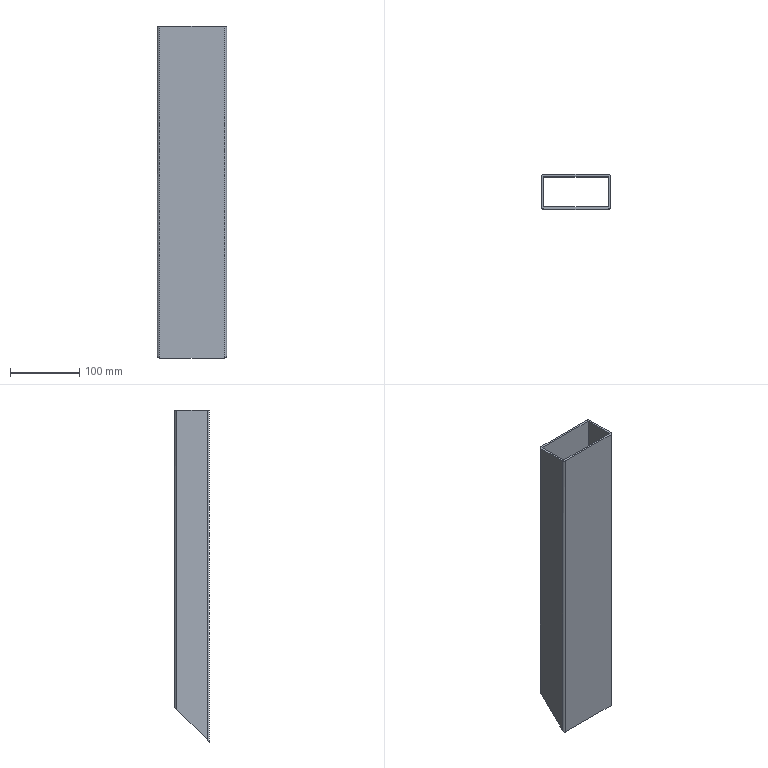Part | SolidWorks | features Extrusion 1, ICE 1 | 1 solid | 18 faces | box 100 x 50 x 480 mm | volume 389136 mm3 | plane 10 | cylinder 8 | commonest cylinder face diameters 0.4 x4 6.4 x4
STEP:
#1=CARTESIAN_POINT('',(-46.8,25.,500.));
#2=VERTEX_POINT('',#1);
#3=CARTESIAN_POINT('',(-46.8,25.,70.));
#4=VERTEX_POINT('',#3);
#5=CARTESIAN_POINT('',(-46.8,25.,500.));
#6=DIRECTION('',(0.,0.,-1.));
#7=VECTOR('',#6,1000.);
#8=LINE('',#5,#7);
#9=EDGE_CURVE('',#2,#4,#8,.T.);
#10=ORIENTED_EDGE('',*,*,#9,.T.);
#11=CARTESIAN_POINT('',(-50.,21.8,66.8));
#12=VERTEX_POINT('',#11);
#13=CARTESIAN_POINT('',(-46.8,25.,70.));
#14=CARTESIAN_POINT('',(-48.675,25.,70.));
#15=CARTESIAN_POINT('',(-50.,23.675,68.675));
#16=CARTESIAN_POINT('',(-50.,21.8,66.8));
#17=(BOUNDED_CURVE()B_SPLINE_CURVE(3,(#13,#14,#15,#16),.UNSPECIFIED.,.F.,.F.)B_SPLINE_CURVE_WITH_KNOTS((4,4),(3.142,4.712),.UNSPECIFIED.)CURVE()GEOMETRIC_REPRESENTATION_ITEM()RATIONAL_B_SPLINE_CURVE((1.,0.8047,0.8047,1.))REPRESENTATION_ITEM(''));
#18=EDGE_CURVE('',#4,#12,#17,.T.);
#19=ORIENTED_EDGE('',*,*,#18,.T.);
#20=CARTESIAN_POINT('',(-50.,21.8,500.));
#21=VERTEX_POINT('',#20);
#22=CARTESIAN_POINT('',(-50.,21.8,500.));
#23=DIRECTION('',(0.,0.,-1.));
#24=VECTOR('',#23,1000.);
#25=LINE('',#22,#24);
#26=EDGE_CURVE('',#21,#12,#25,.T.);
#27=ORIENTED_EDGE('',*,*,#26,.F.);
#28=CARTESIAN_POINT('',(-46.8,21.8,500.));
#29=DIRECTION('',(0.,0.,1.));
#30=DIRECTION('',(1.,0.,0.));
#31=AXIS2_PLACEMENT_3D('',#28,#29,#30);
#32=CIRCLE('',#31,3.2);
#33=EDGE_CURVE('',#2,#21,#32,.T.);
#34=ORIENTED_EDGE('',*,*,#33,.F.);
#35=EDGE_LOOP('',(#10,#19,#27,#34));
#36=FACE_OUTER_BOUND('',#35,.T.);
#37=CARTESIAN_POINT('',(-46.8,21.8,500.));
#38=DIRECTION('',(0.,0.,-1.));
#39=DIRECTION('',(-1.,0.,0.));
#40=AXIS2_PLACEMENT_3D('',#37,#38,#39);
#41=CYLINDRICAL_SURFACE('',#40,3.2);
#42=ADVANCED_FACE('',(#36),#41,.T.);
#43=ORIENTED_EDGE('',*,*,#26,.T.);
#44=CARTESIAN_POINT('',(-50.,-21.8,23.2));
#45=VERTEX_POINT('',#44);
#46=CARTESIAN_POINT('',(-50.,238.4,283.4));
#47=DIRECTION('',(0.,-0.7071,-0.7071));
#48=VECTOR('',#47,1000.);
#49=LINE('',#46,#48);
#50=EDGE_CURVE('',#12,#45,#49,.T.);
#51=ORIENTED_EDGE('',*,*,#50,.T.);
#52=CARTESIAN_POINT('',(-50.,-21.8,500.));
#53=VERTEX_POINT('',#52);
#54=CARTESIAN_POINT('',(-50.,-21.8,500.));
#55=DIRECTION('',(0.,0.,-1.));
#56=VECTOR('',#55,1000.);
#57=LINE('',#54,#56);
#58=EDGE_CURVE('',#53,#45,#57,.T.);
#59=ORIENTED_EDGE('',*,*,#58,.F.);
#60=CARTESIAN_POINT('',(-50.,21.8,500.));
#61=DIRECTION('',(0.,-1.,0.));
#62=VECTOR('',#61,1000.);
#63=LINE('',#60,#62);
#64=EDGE_CURVE('',#21,#53,#63,.T.);
#65=ORIENTED_EDGE('',*,*,#64,.F.);
#66=EDGE_LOOP('',(#43,#51,#59,#65));
#67=FACE_OUTER_BOUND('',#66,.T.);
#68=CARTESIAN_POINT('',(-50.,21.8,500.));
#69=DIRECTION('',(1.,0.,0.));
#70=DIRECTION('',(0.,1.,0.));
#71=AXIS2_PLACEMENT_3D('',#68,#69,#70);
#72=PLANE('',#71);
#73=ADVANCED_FACE('',(#67),#72,.F.);
#74=ORIENTED_EDGE('',*,*,#58,.T.);
#75=CARTESIAN_POINT('',(-46.8,-25.,20.));
#76=VERTEX_POINT('',#75);
#77=CARTESIAN_POINT('',(-50.,-21.8,23.2));
#78=CARTESIAN_POINT('',(-50.,-23.675,21.325));
#79=CARTESIAN_POINT('',(-48.675,-25.,20.));
#80=CARTESIAN_POINT('',(-46.8,-25.,20.));
#81=(BOUNDED_CURVE()B_SPLINE_CURVE(3,(#77,#78,#79,#80),.UNSPECIFIED.,.F.,.F.)B_SPLINE_CURVE_WITH_KNOTS((4,4),(4.712,6.283),.UNSPECIFIED.)CURVE()GEOMETRIC_REPRESENTATION_ITEM()RATIONAL_B_SPLINE_CURVE((1.,0.8047,0.8047,1.))REPRESENTATION_ITEM(''));
#82=EDGE_CURVE('',#45,#76,#81,.T.);
#83=ORIENTED_EDGE('',*,*,#82,.T.);
#84=CARTESIAN_POINT('',(-46.8,-25.,500.));
#85=VERTEX_POINT('',#84);
#86=CARTESIAN_POINT('',(-46.8,-25.,500.));
#87=DIRECTION('',(0.,0.,-1.));
#88=VECTOR('',#87,1000.);
#89=LINE('',#86,#88);
#90=EDGE_CURVE('',#85,#76,#89,.T.);
#91=ORIENTED_EDGE('',*,*,#90,.F.);
#92=CARTESIAN_POINT('',(-46.8,-21.8,500.));
#93=DIRECTION('',(0.,0.,1.));
#94=DIRECTION('',(1.,0.,0.));
#95=AXIS2_PLACEMENT_3D('',#92,#93,#94);
#96=CIRCLE('',#95,3.2);
#97=EDGE_CURVE('',#53,#85,#96,.T.);
#98=ORIENTED_EDGE('',*,*,#97,.F.);
#99=EDGE_LOOP('',(#74,#83,#91,#98));
#100=FACE_OUTER_BOUND('',#99,.T.);
#101=CARTESIAN_POINT('',(-46.8,-21.8,500.));
#102=DIRECTION('',(0.,0.,-1.));
#103=DIRECTION('',(-1.,0.,0.));
#104=AXIS2_PLACEMENT_3D('',#101,#102,#103);
#105=CYLINDRICAL_SURFACE('',#104,3.2);
#106=ADVANCED_FACE('',(#100),#105,.T.);
#107=ORIENTED_EDGE('',*,*,#90,.T.);
#108=CARTESIAN_POINT('',(46.8,-25.,20.));
#109=VERTEX_POINT('',#108);
#110=CARTESIAN_POINT('',(-430.,-25.,20.));
#111=DIRECTION('',(1.,0.,0.));
#112=VECTOR('',#111,1000.);
#113=LINE('',#110,#112);
#114=EDGE_CURVE('',#76,#109,#113,.T.);
#115=ORIENTED_EDGE('',*,*,#114,.T.);
#116=CARTESIAN_POINT('',(46.8,-25.,500.));
#117=VERTEX_POINT('',#116);
#118=CARTESIAN_POINT('',(46.8,-25.,500.));
#119=DIRECTION('',(0.,0.,-1.));
#120=VECTOR('',#119,1000.);
#121=LINE('',#118,#120);
#122=EDGE_CURVE('',#117,#109,#121,.T.);
#123=ORIENTED_EDGE('',*,*,#122,.F.);
#124=CARTESIAN_POINT('',(-46.8,-25.,500.));
#125=DIRECTION('',(1.,0.,0.));
#126=VECTOR('',#125,1000.);
#127=LINE('',#124,#126);
#128=EDGE_CURVE('',#85,#117,#127,.T.);
#129=ORIENTED_EDGE('',*,*,#128,.F.);
#130=EDGE_LOOP('',(#107,#115,#123,#129));
#131=FACE_OUTER_BOUND('',#130,.T.);
#132=CARTESIAN_POINT('',(-46.8,-25.,500.));
#133=DIRECTION('',(0.,1.,0.));
#134=DIRECTION('',(0.,0.,1.));
#135=AXIS2_PLACEMENT_3D('',#132,#133,#134);
#136=PLANE('',#135);
#137=ADVANCED_FACE('',(#131),#136,.F.);
#138=ORIENTED_EDGE('',*,*,#122,.T.);
#139=CARTESIAN_POINT('',(50.,-21.8,23.2));
#140=VERTEX_POINT('',#139);
#141=CARTESIAN_POINT('',(46.8,-25.,20.));
#142=CARTESIAN_POINT('',(48.675,-25.,20.));
#143=CARTESIAN_POINT('',(50.,-23.675,21.325));
#144=CARTESIAN_POINT('',(50.,-21.8,23.2));
#145=(BOUNDED_CURVE()B_SPLINE_CURVE(3,(#141,#142,#143,#144),.UNSPECIFIED.,.F.,.F.)B_SPLINE_CURVE_WITH_KNOTS((4,4),(0.,1.571),.UNSPECIFIED.)CURVE()GEOMETRIC_REPRESENTATION_ITEM()RATIONAL_B_SPLINE_CURVE((1.,0.8047,0.8047,1.))REPRESENTATION_ITEM(''));
#146=EDGE_CURVE('',#109,#140,#145,.T.);
#147=ORIENTED_EDGE('',*,*,#146,.T.);
#148=CARTESIAN_POINT('',(50.,-21.8,500.));
#149=VERTEX_POINT('',#148);
#150=CARTESIAN_POINT('',(50.,-21.8,500.));
#151=DIRECTION('',(0.,0.,-1.));
#152=VECTOR('',#151,1000.);
#153=LINE('',#150,#152);
#154=EDGE_CURVE('',#149,#140,#153,.T.);
#155=ORIENTED_EDGE('',*,*,#154,.F.);
#156=CARTESIAN_POINT('',(46.8,-21.8,500.));
#157=DIRECTION('',(0.,0.,1.));
#158=DIRECTION('',(1.,0.,0.));
#159=AXIS2_PLACEMENT_3D('',#156,#157,#158);
#160=CIRCLE('',#159,3.2);
#161=EDGE_CURVE('',#117,#149,#160,.T.);
#162=ORIENTED_EDGE('',*,*,#161,.F.);
#163=EDGE_LOOP('',(#138,#147,#155,#162));
#164=FACE_OUTER_BOUND('',#163,.T.);
#165=CARTESIAN_POINT('',(46.8,-21.8,500.));
#166=DIRECTION('',(0.,0.,-1.));
#167=DIRECTION('',(-1.,0.,0.));
#168=AXIS2_PLACEMENT_3D('',#165,#166,#167);
#169=CYLINDRICAL_SURFACE('',#168,3.2);
#170=ADVANCED_FACE('',(#164),#169,.T.);
#171=CARTESIAN_POINT('',(50.,21.8,66.8));
#172=VERTEX_POINT('',#171);
#173=CARTESIAN_POINT('',(50.,25.,70.));
#174=DIRECTION('',(0.,-0.7071,-0.7071));
#175=VECTOR('',#174,1000.);
#176=LINE('',#173,#175);
#177=EDGE_CURVE('',#172,#140,#176,.T.);
#178=ORIENTED_EDGE('',*,*,#177,.F.);
#179=CARTESIAN_POINT('',(50.,21.8,500.));
#180=VERTEX_POINT('',#179);
#181=CARTESIAN_POINT('',(50.,21.8,500.));
#182=DIRECTION('',(0.,0.,-1.));
#183=VECTOR('',#182,1000.);
#184=LINE('',#181,#183);
#185=EDGE_CURVE('',#180,#172,#184,.T.);
#186=ORIENTED_EDGE('',*,*,#185,.F.);
#187=CARTESIAN_POINT('',(50.,21.8,500.));
#188=DIRECTION('',(0.,-1.,0.));
#189=VECTOR('',#188,1000.);
#190=LINE('',#187,#189);
#191=EDGE_CURVE('',#180,#149,#190,.T.);
#192=ORIENTED_EDGE('',*,*,#191,.T.);
#193=ORIENTED_EDGE('',*,*,#154,.T.);
#194=EDGE_LOOP('',(#178,#186,#192,#193));
#195=FACE_OUTER_BOUND('',#194,.T.);
#196=CARTESIAN_POINT('',(50.,21.8,500.));
#197=DIRECTION('',(1.,0.,0.));
#198=DIRECTION('',(0.,1.,0.));
#199=AXIS2_PLACEMENT_3D('',#196,#197,#198);
#200=PLANE('',#199);
#201=ADVANCED_FACE('',(#195),#200,.T.);
#202=CARTESIAN_POINT('',(46.8,25.,70.));
#203=VERTEX_POINT('',#202);
#204=CARTESIAN_POINT('',(46.8,25.,70.));
#205=CARTESIAN_POINT('',(48.675,25.,70.));
#206=CARTESIAN_POINT('',(50.,23.675,68.675));
#207=CARTESIAN_POINT('',(50.,21.8,66.8));
#208=(BOUNDED_CURVE()B_SPLINE_CURVE(3,(#204,#205,#206,#207),.UNSPECIFIED.,.F.,.F.)B_SPLINE_CURVE_WITH_KNOTS((4,4),(3.142,4.712),.UNSPECIFIED.)CURVE()GEOMETRIC_REPRESENTATION_ITEM()RATIONAL_B_SPLINE_CURVE((1.,0.8047,0.8047,1.))REPRESENTATION_ITEM(''));
#209=EDGE_CURVE('',#203,#172,#208,.T.);
#210=ORIENTED_EDGE('',*,*,#209,.F.);
#211=CARTESIAN_POINT('',(46.8,25.,500.));
#212=VERTEX_POINT('',#211);
#213=CARTESIAN_POINT('',(46.8,25.,500.));
#214=DIRECTION('',(0.,0.,-1.));
#215=VECTOR('',#214,1000.);
#216=LINE('',#213,#215);
#217=EDGE_CURVE('',#212,#203,#216,.T.);
#218=ORIENTED_EDGE('',*,*,#217,.F.);
#219=CARTESIAN_POINT('',(46.8,21.8,500.));
#220=DIRECTION('',(0.,0.,-1.));
#221=DIRECTION('',(-1.,0.,0.));
#222=AXIS2_PLACEMENT_3D('',#219,#220,#221);
#223=CIRCLE('',#222,3.2);
#224=EDGE_CURVE('',#212,#180,#223,.T.);
#225=ORIENTED_EDGE('',*,*,#224,.T.);
#226=ORIENTED_EDGE('',*,*,#185,.T.);
#227=EDGE_LOOP('',(#210,#218,#225,#226));
#228=FACE_OUTER_BOUND('',#227,.T.);
#229=CARTESIAN_POINT('',(46.8,21.8,500.));
#230=DIRECTION('',(0.,0.,-1.));
#231=DIRECTION('',(-1.,0.,0.));
#232=AXIS2_PLACEMENT_3D('',#229,#230,#231);
#233=CYLINDRICAL_SURFACE('',#232,3.2);
#234=ADVANCED_FACE('',(#228),#233,.T.);
#235=CARTESIAN_POINT('',(-430.,25.,70.));
#236=DIRECTION('',(1.,0.,0.));
#237=VECTOR('',#236,1000.);
#238=LINE('',#235,#237);
#239=EDGE_CURVE('',#4,#203,#238,.T.);
#240=ORIENTED_EDGE('',*,*,#239,.F.);
#241=ORIENTED_EDGE('',*,*,#9,.F.);
#242=CARTESIAN_POINT('',(-46.8,25.,500.));
#243=DIRECTION('',(1.,0.,0.));
#244=VECTOR('',#243,1000.);
#245=LINE('',#242,#244);
#246=EDGE_CURVE('',#2,#212,#245,.T.);
#247=ORIENTED_EDGE('',*,*,#246,.T.);
#248=ORIENTED_EDGE('',*,*,#217,.T.);
#249=EDGE_LOOP('',(#240,#241,#247,#248));
#250=FACE_OUTER_BOUND('',#249,.T.);
#251=CARTESIAN_POINT('',(-46.8,25.,500.));
#252=DIRECTION('',(0.,1.,0.));
#253=DIRECTION('',(0.,0.,1.));
#254=AXIS2_PLACEMENT_3D('',#251,#252,#253);
#255=PLANE('',#254);
#256=ADVANCED_FACE('',(#250),#255,.T.);
#257=CARTESIAN_POINT('',(-46.8,22.,500.));
#258=VERTEX_POINT('',#257);
#259=CARTESIAN_POINT('',(46.8,22.,500.));
#260=VERTEX_POINT('',#259);
#261=CARTESIAN_POINT('',(0.,22.,500.));
#262=DIRECTION('',(1.,0.,0.));
#263=VECTOR('',#262,1000.);
#264=LINE('',#261,#263);
#265=EDGE_CURVE('',#258,#260,#264,.T.);
#266=ORIENTED_EDGE('',*,*,#265,.T.);
#267=CARTESIAN_POINT('',(47.,21.8,500.));
#268=VERTEX_POINT('',#267);
#269=CARTESIAN_POINT('',(46.8,21.8,500.));
#270=DIRECTION('',(0.,0.,-1.));
#271=DIRECTION('',(1.,0.,0.));
#272=AXIS2_PLACEMENT_3D('',#269,#270,#271);
#273=CIRCLE('',#272,0.2);
#274=EDGE_CURVE('',#260,#268,#273,.T.);
#275=ORIENTED_EDGE('',*,*,#274,.T.);
#276=CARTESIAN_POINT('',(47.,-21.8,500.));
#277=VERTEX_POINT('',#276);
#278=CARTESIAN_POINT('',(47.,0.,500.));
#279=DIRECTION('',(0.,-1.,0.));
#280=VECTOR('',#279,1000.);
#281=LINE('',#278,#280);
#282=EDGE_CURVE('',#268,#277,#281,.T.);
#283=ORIENTED_EDGE('',*,*,#282,.T.);
#284=CARTESIAN_POINT('',(46.8,-22.,500.));
#285=VERTEX_POINT('',#284);
#286=CARTESIAN_POINT('',(46.8,-21.8,500.));
#287=DIRECTION('',(0.,0.,-1.));
#288=DIRECTION('',(1.,0.,0.));
#289=AXIS2_PLACEMENT_3D('',#286,#287,#288);
#290=CIRCLE('',#289,0.2);
#291=EDGE_CURVE('',#277,#285,#290,.T.);
#292=ORIENTED_EDGE('',*,*,#291,.T.);
#293=CARTESIAN_POINT('',(-46.8,-22.,500.));
#294=VERTEX_POINT('',#293);
#295=CARTESIAN_POINT('',(0.,-22.,500.));
#296=DIRECTION('',(1.,0.,0.));
#297=VECTOR('',#296,1000.);
#298=LINE('',#295,#297);
#299=EDGE_CURVE('',#294,#285,#298,.T.);
#300=ORIENTED_EDGE('',*,*,#299,.F.);
#301=CARTESIAN_POINT('',(-47.,-21.8,500.));
#302=VERTEX_POINT('',#301);
#303=CARTESIAN_POINT('',(-46.8,-21.8,500.));
#304=DIRECTION('',(0.,0.,-1.));
#305=DIRECTION('',(1.,0.,0.));
#306=AXIS2_PLACEMENT_3D('',#303,#304,#305);
#307=CIRCLE('',#306,0.2);
#308=EDGE_CURVE('',#294,#302,#307,.T.);
#309=ORIENTED_EDGE('',*,*,#308,.T.);
#310=CARTESIAN_POINT('',(-47.,21.8,500.));
#311=VERTEX_POINT('',#310);
#312=CARTESIAN_POINT('',(-47.,0.,500.));
#313=DIRECTION('',(0.,-1.,0.));
#314=VECTOR('',#313,1000.);
#315=LINE('',#312,#314);
#316=EDGE_CURVE('',#311,#302,#315,.T.);
#317=ORIENTED_EDGE('',*,*,#316,.F.);
#318=CARTESIAN_POINT('',(-46.8,21.8,500.));
#319=DIRECTION('',(0.,0.,1.));
#320=DIRECTION('',(1.,0.,0.));
#321=AXIS2_PLACEMENT_3D('',#318,#319,#320);
#322=CIRCLE('',#321,0.2);
#323=EDGE_CURVE('',#258,#311,#322,.T.);
#324=ORIENTED_EDGE('',*,*,#323,.F.);
#325=EDGE_LOOP('',(#266,#275,#283,#292,#300,#309,#317,#324));
#326=FACE_BOUND('',#325,.T.);
#327=ORIENTED_EDGE('',*,*,#33,.T.);
#328=ORIENTED_EDGE('',*,*,#64,.T.);
#329=ORIENTED_EDGE('',*,*,#97,.T.);
#330=ORIENTED_EDGE('',*,*,#128,.T.);
#331=ORIENTED_EDGE('',*,*,#161,.T.);
#332=ORIENTED_EDGE('',*,*,#191,.F.);
#333=ORIENTED_EDGE('',*,*,#224,.F.);
#334=ORIENTED_EDGE('',*,*,#246,.F.);
#335=EDGE_LOOP('',(#327,#328,#329,#330,#331,#332,#333,#334));
#336=FACE_OUTER_BOUND('',#335,.T.);
#337=CARTESIAN_POINT('',(-46.8,21.8,500.));
#338=DIRECTION('',(0.,0.,1.));
#339=DIRECTION('',(1.,0.,0.));
#340=AXIS2_PLACEMENT_3D('',#337,#338,#339);
#341=PLANE('',#340);
#342=ADVANCED_FACE('',(#326,#336),#341,.T.);
#343=CARTESIAN_POINT('',(-46.8,22.,67.));
#344=VERTEX_POINT('',#343);
#345=CARTESIAN_POINT('',(-46.8,22.,500.));
#346=DIRECTION('',(0.,0.,-1.));
#347=VECTOR('',#346,1000.);
#348=LINE('',#345,#347);
#349=EDGE_CURVE('',#258,#344,#348,.T.);
#350=ORIENTED_EDGE('',*,*,#349,.T.);
#351=CARTESIAN_POINT('',(46.8,22.,67.));
#352=VERTEX_POINT('',#351);
#353=CARTESIAN_POINT('',(0.,22.,67.));
#354=DIRECTION('',(1.,0.,0.));
#355=VECTOR('',#354,1000.);
#356=LINE('',#353,#355);
#357=EDGE_CURVE('',#344,#352,#356,.T.);
#358=ORIENTED_EDGE('',*,*,#357,.T.);
#359=CARTESIAN_POINT('',(46.8,22.,500.));
#360=DIRECTION('',(0.,0.,-1.));
#361=VECTOR('',#360,1000.);
#362=LINE('',#359,#361);
#363=EDGE_CURVE('',#260,#352,#362,.T.);
#364=ORIENTED_EDGE('',*,*,#363,.F.);
#365=ORIENTED_EDGE('',*,*,#265,.F.);
#366=EDGE_LOOP('',(#350,#358,#364,#365));
#367=FACE_OUTER_BOUND('',#366,.T.);
#368=CARTESIAN_POINT('',(0.,22.,500.));
#369=DIRECTION('',(0.,1.,0.));
#370=DIRECTION('',(0.,0.,1.));
#371=AXIS2_PLACEMENT_3D('',#368,#369,#370);
#372=PLANE('',#371);
#373=ADVANCED_FACE('',(#367),#372,.F.);
#374=CARTESIAN_POINT('',(-47.,21.8,66.8));
#375=VERTEX_POINT('',#374);
#376=CARTESIAN_POINT('',(-46.8,22.,67.));
#377=CARTESIAN_POINT('',(-46.917,22.,67.));
#378=CARTESIAN_POINT('',(-47.,21.917,66.917));
#379=CARTESIAN_POINT('',(-47.,21.8,66.8));
#380=(BOUNDED_CURVE()B_SPLINE_CURVE(3,(#376,#377,#378,#379),.UNSPECIFIED.,.F.,.T.)B_SPLINE_CURVE_WITH_KNOTS((4,4),(3.142,4.712),.UNSPECIFIED.)CURVE()GEOMETRIC_REPRESENTATION_ITEM()RATIONAL_B_SPLINE_CURVE((1.,0.8047,0.8047,1.))REPRESENTATION_ITEM(''));
#381=EDGE_CURVE('',#344,#375,#380,.T.);
#382=ORIENTED_EDGE('',*,*,#381,.F.);
#383=ORIENTED_EDGE('',*,*,#349,.F.);
#384=ORIENTED_EDGE('',*,*,#323,.T.);
#385=CARTESIAN_POINT('',(-47.,21.8,500.));
#386=DIRECTION('',(0.,0.,-1.));
#387=VECTOR('',#386,1000.);
#388=LINE('',#385,#387);
#389=EDGE_CURVE('',#311,#375,#388,.T.);
#390=ORIENTED_EDGE('',*,*,#389,.T.);
#391=EDGE_LOOP('',(#382,#383,#384,#390));
#392=FACE_OUTER_BOUND('',#391,.T.);
#393=CARTESIAN_POINT('',(-46.8,21.8,500.));
#394=DIRECTION('',(0.,0.,-1.));
#395=DIRECTION('',(-1.,0.,0.));
#396=AXIS2_PLACEMENT_3D('',#393,#394,#395);
#397=CYLINDRICAL_SURFACE('',#396,0.2);
#398=ADVANCED_FACE('',(#392),#397,.F.);
#399=CARTESIAN_POINT('',(-47.,-21.8,23.2));
#400=VERTEX_POINT('',#399);
#401=CARTESIAN_POINT('',(-47.,227.5,272.5));
#402=DIRECTION('',(0.,-0.7071,-0.7071));
#403=VECTOR('',#402,1000.);
#404=LINE('',#401,#403);
#405=EDGE_CURVE('',#375,#400,#404,.T.);
#406=ORIENTED_EDGE('',*,*,#405,.F.);
#407=ORIENTED_EDGE('',*,*,#389,.F.);
#408=ORIENTED_EDGE('',*,*,#316,.T.);
#409=CARTESIAN_POINT('',(-47.,-21.8,500.));
#410=DIRECTION('',(0.,0.,-1.));
#411=VECTOR('',#410,1000.);
#412=LINE('',#409,#411);
#413=EDGE_CURVE('',#302,#400,#412,.T.);
#414=ORIENTED_EDGE('',*,*,#413,.T.);
#415=EDGE_LOOP('',(#406,#407,#408,#414));
#416=FACE_OUTER_BOUND('',#415,.T.);
#417=CARTESIAN_POINT('',(-47.,0.,500.));
#418=DIRECTION('',(1.,0.,0.));
#419=DIRECTION('',(0.,1.,0.));
#420=AXIS2_PLACEMENT_3D('',#417,#418,#419);
#421=PLANE('',#420);
#422=ADVANCED_FACE('',(#416),#421,.T.);
#423=CARTESIAN_POINT('',(-46.8,-22.,23.));
#424=VERTEX_POINT('',#423);
#425=CARTESIAN_POINT('',(-46.8,-22.,500.));
#426=DIRECTION('',(0.,0.,-1.));
#427=VECTOR('',#426,1000.);
#428=LINE('',#425,#427);
#429=EDGE_CURVE('',#294,#424,#428,.T.);
#430=ORIENTED_EDGE('',*,*,#429,.T.);
#431=CARTESIAN_POINT('',(-46.8,-22.,23.));
#432=CARTESIAN_POINT('',(-46.917,-22.,23.));
#433=CARTESIAN_POINT('',(-47.,-21.917,23.083));
#434=CARTESIAN_POINT('',(-47.,-21.8,23.2));
#435=(BOUNDED_CURVE()B_SPLINE_CURVE(3,(#431,#432,#433,#434),.UNSPECIFIED.,.F.,.F.)B_SPLINE_CURVE_WITH_KNOTS((4,4),(0.,1.571),.UNSPECIFIED.)CURVE()GEOMETRIC_REPRESENTATION_ITEM()RATIONAL_B_SPLINE_CURVE((1.,0.8047,0.8047,1.))REPRESENTATION_ITEM(''));
#436=EDGE_CURVE('',#424,#400,#435,.T.);
#437=ORIENTED_EDGE('',*,*,#436,.T.);
#438=ORIENTED_EDGE('',*,*,#413,.F.);
#439=ORIENTED_EDGE('',*,*,#308,.F.);
#440=EDGE_LOOP('',(#430,#437,#438,#439));
#441=FACE_OUTER_BOUND('',#440,.T.);
#442=CARTESIAN_POINT('',(-46.8,-21.8,500.));
#443=DIRECTION('',(0.,0.,-1.));
#444=DIRECTION('',(-1.,0.,0.));
#445=AXIS2_PLACEMENT_3D('',#442,#443,#444);
#446=CYLINDRICAL_SURFACE('',#445,0.2);
#447=ADVANCED_FACE('',(#441),#446,.F.);
#448=CARTESIAN_POINT('',(46.8,-22.,23.));
#449=VERTEX_POINT('',#448);
#450=CARTESIAN_POINT('',(0.,-22.,23.));
#451=DIRECTION('',(1.,0.,0.));
#452=VECTOR('',#451,1000.);
#453=LINE('',#450,#452);
#454=EDGE_CURVE('',#424,#449,#453,.T.);
#455=ORIENTED_EDGE('',*,*,#454,.F.);
#456=ORIENTED_EDGE('',*,*,#429,.F.);
#457=ORIENTED_EDGE('',*,*,#299,.T.);
#458=CARTESIAN_POINT('',(46.8,-22.,500.));
#459=DIRECTION('',(0.,0.,-1.));
#460=VECTOR('',#459,1000.);
#461=LINE('',#458,#460);
#462=EDGE_CURVE('',#285,#449,#461,.T.);
#463=ORIENTED_EDGE('',*,*,#462,.T.);
#464=EDGE_LOOP('',(#455,#456,#457,#463));
#465=FACE_OUTER_BOUND('',#464,.T.);
#466=CARTESIAN_POINT('',(0.,-22.,500.));
#467=DIRECTION('',(0.,1.,0.));
#468=DIRECTION('',(0.,0.,1.));
#469=AXIS2_PLACEMENT_3D('',#466,#467,#468);
#470=PLANE('',#469);
#471=ADVANCED_FACE('',(#465),#470,.T.);
#472=CARTESIAN_POINT('',(47.,-21.8,23.2));
#473=VERTEX_POINT('',#472);
#474=CARTESIAN_POINT('',(47.,-21.8,500.));
#475=DIRECTION('',(0.,0.,-1.));
#476=VECTOR('',#475,1000.);
#477=LINE('',#474,#476);
#478=EDGE_CURVE('',#277,#473,#477,.T.);
#479=ORIENTED_EDGE('',*,*,#478,.T.);
#480=CARTESIAN_POINT('',(47.,-21.8,23.2));
#481=CARTESIAN_POINT('',(47.,-21.917,23.083));
#482=CARTESIAN_POINT('',(46.917,-22.,23.));
#483=CARTESIAN_POINT('',(46.8,-22.,23.));
#484=(BOUNDED_CURVE()B_SPLINE_CURVE(3,(#480,#481,#482,#483),.UNSPECIFIED.,.F.,.F.)B_SPLINE_CURVE_WITH_KNOTS((4,4),(4.712,6.283),.UNSPECIFIED.)CURVE()GEOMETRIC_REPRESENTATION_ITEM()RATIONAL_B_SPLINE_CURVE((1.,0.8047,0.8047,1.))REPRESENTATION_ITEM(''));
#485=EDGE_CURVE('',#473,#449,#484,.T.);
#486=ORIENTED_EDGE('',*,*,#485,.T.);
#487=ORIENTED_EDGE('',*,*,#462,.F.);
#488=ORIENTED_EDGE('',*,*,#291,.F.);
#489=EDGE_LOOP('',(#479,#486,#487,#488));
#490=FACE_OUTER_BOUND('',#489,.T.);
#491=CARTESIAN_POINT('',(46.8,-21.8,500.));
#492=DIRECTION('',(0.,0.,-1.));
#493=DIRECTION('',(-1.,0.,0.));
#494=AXIS2_PLACEMENT_3D('',#491,#492,#493);
#495=CYLINDRICAL_SURFACE('',#494,0.2);
#496=ADVANCED_FACE('',(#490),#495,.F.);
#497=CARTESIAN_POINT('',(47.,21.8,66.8));
#498=VERTEX_POINT('',#497);
#499=CARTESIAN_POINT('',(47.,21.8,500.));
#500=DIRECTION('',(0.,0.,-1.));
#501=VECTOR('',#500,1000.);
#502=LINE('',#499,#501);
#503=EDGE_CURVE('',#268,#498,#502,.T.);
#504=ORIENTED_EDGE('',*,*,#503,.T.);
#505=CARTESIAN_POINT('',(47.,227.5,272.5));
#506=DIRECTION('',(0.,-0.7071,-0.7071));
#507=VECTOR('',#506,1000.);
#508=LINE('',#505,#507);
#509=EDGE_CURVE('',#498,#473,#508,.T.);
#510=ORIENTED_EDGE('',*,*,#509,.T.);
#511=ORIENTED_EDGE('',*,*,#478,.F.);
#512=ORIENTED_EDGE('',*,*,#282,.F.);
#513=EDGE_LOOP('',(#504,#510,#511,#512));
#514=FACE_OUTER_BOUND('',#513,.T.);
#515=CARTESIAN_POINT('',(47.,0.,500.));
#516=DIRECTION('',(1.,0.,0.));
#517=DIRECTION('',(0.,1.,0.));
#518=AXIS2_PLACEMENT_3D('',#515,#516,#517);
#519=PLANE('',#518);
#520=ADVANCED_FACE('',(#514),#519,.F.);
#521=ORIENTED_EDGE('',*,*,#363,.T.);
#522=CARTESIAN_POINT('',(46.8,22.,67.));
#523=CARTESIAN_POINT('',(46.917,22.,67.));
#524=CARTESIAN_POINT('',(47.,21.917,66.917));
#525=CARTESIAN_POINT('',(47.,21.8,66.8));
#526=(BOUNDED_CURVE()B_SPLINE_CURVE(3,(#522,#523,#524,#525),.UNSPECIFIED.,.F.,.F.)B_SPLINE_CURVE_WITH_KNOTS((4,4),(3.142,4.712),.UNSPECIFIED.)CURVE()GEOMETRIC_REPRESENTATION_ITEM()RATIONAL_B_SPLINE_CURVE((1.,0.8047,0.8047,1.))REPRESENTATION_ITEM(''));
#527=EDGE_CURVE('',#352,#498,#526,.T.);
#528=ORIENTED_EDGE('',*,*,#527,.T.);
#529=ORIENTED_EDGE('',*,*,#503,.F.);
#530=ORIENTED_EDGE('',*,*,#274,.F.);
#531=EDGE_LOOP('',(#521,#528,#529,#530));
#532=FACE_OUTER_BOUND('',#531,.T.);
#533=CARTESIAN_POINT('',(46.8,21.8,500.));
#534=DIRECTION('',(0.,0.,-1.));
#535=DIRECTION('',(-1.,0.,0.));
#536=AXIS2_PLACEMENT_3D('',#533,#534,#535);
#537=CYLINDRICAL_SURFACE('',#536,0.2);
#538=ADVANCED_FACE('',(#532),#537,.F.);
#539=ORIENTED_EDGE('',*,*,#381,.T.);
#540=ORIENTED_EDGE('',*,*,#405,.T.);
#541=ORIENTED_EDGE('',*,*,#436,.F.);
#542=ORIENTED_EDGE('',*,*,#454,.T.);
#543=ORIENTED_EDGE('',*,*,#485,.F.);
#544=ORIENTED_EDGE('',*,*,#509,.F.);
#545=ORIENTED_EDGE('',*,*,#527,.F.);
#546=ORIENTED_EDGE('',*,*,#357,.F.);
#547=EDGE_LOOP('',(#539,#540,#541,#542,#543,#544,#545,#546));
#548=FACE_BOUND('',#547,.T.);
#549=ORIENTED_EDGE('',*,*,#239,.T.);
#550=ORIENTED_EDGE('',*,*,#209,.T.);
#551=ORIENTED_EDGE('',*,*,#177,.T.);
#552=ORIENTED_EDGE('',*,*,#146,.F.);
#553=ORIENTED_EDGE('',*,*,#114,.F.);
#554=ORIENTED_EDGE('',*,*,#82,.F.);
#555=ORIENTED_EDGE('',*,*,#50,.F.);
#556=ORIENTED_EDGE('',*,*,#18,.F.);
#557=EDGE_LOOP('',(#549,#550,#551,#552,#553,#554,#555,#556));
#558=FACE_OUTER_BOUND('',#557,.T.);
#559=CARTESIAN_POINT('',(-430.,25.,70.));
#560=DIRECTION('',(0.,-0.7071,0.7071));
#561=DIRECTION('',(0.,-0.7071,-0.7071));
#562=AXIS2_PLACEMENT_3D('',#559,#560,#561);
#563=PLANE('',#562);
#564=ADVANCED_FACE('',(#548,#558),#563,.F.);
#565=CLOSED_SHELL('',(#42,#73,#106,#137,#170,#201,#234,#256,#342,#373,#398,#422,#447,#471,#496,#520,#538,#564));
#566=MANIFOLD_SOLID_BREP('',#565);
#567=CARTESIAN_POINT('',(0.,0.,0.));
#568=DIRECTION('',(0.,0.,1.));
#569=DIRECTION('',(1.,0.,0.));
#570=AXIS2_PLACEMENT_3D('',#567,#568,#569);
#571=(LENGTH_UNIT()NAMED_UNIT(*)SI_UNIT(.MILLI.,.METRE.));
#572=UNCERTAINTY_MEASURE_WITH_UNIT(LENGTH_MEASURE(0.00001),#571,'','');
#573=(NAMED_UNIT(*)PLANE_ANGLE_UNIT()SI_UNIT($,.RADIAN.));
#574=(NAMED_UNIT(*)SI_UNIT($,.STERADIAN.)SOLID_ANGLE_UNIT());
#575=(GEOMETRIC_REPRESENTATION_CONTEXT(3)GLOBAL_UNCERTAINTY_ASSIGNED_CONTEXT((#572))GLOBAL_UNIT_ASSIGNED_CONTEXT((#571,#573,#574))REPRESENTATION_CONTEXT('',''));
#576=ADVANCED_BREP_SHAPE_REPRESENTATION('',(#566,#570),#575);